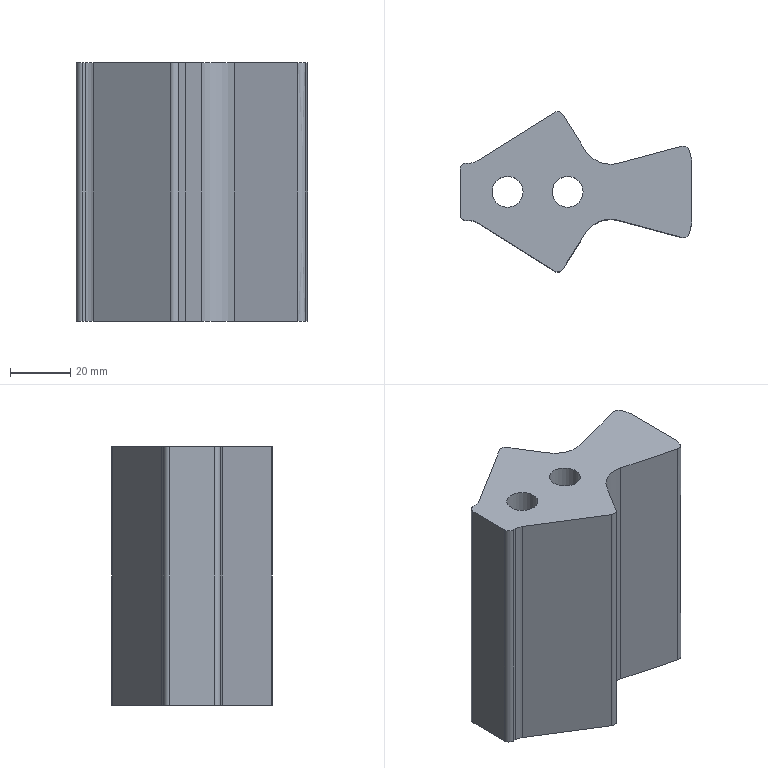Part | NX | features solid 2 | 1 solid | 34 faces | box 77 x 53.346 x 86 mm | volume 174595 mm3 | cylinder 14 | plane 14 | spline 6 | commonest cylinder face diameters 4 x4 10 x4 10.3 x2 17 x2 20 x2
STEP:
#1=CARTESIAN_POINT('',(1558.616,0.,32.));
#2=VERTEX_POINT('',#1);
#3=CARTESIAN_POINT('',(1567.116,0.,32.));
#4=DIRECTION('',(0.,0.,-1.));
#5=DIRECTION('',(-1.,0.,0.));
#6=AXIS2_PLACEMENT_3D('',#3,#4,#5);
#7=CIRCLE('',#6,8.5);
#8=EDGE_CURVE('',#2,#2,#7,.T.);
#9=ORIENTED_EDGE('',*,*,#8,.F.);
#10=EDGE_LOOP('',(#9));
#11=FACE_BOUND('',#10,.T.);
#12=CARTESIAN_POINT('',(1558.616,0.,-8.));
#13=VERTEX_POINT('',#12);
#14=CARTESIAN_POINT('',(1567.116,0.,-8.));
#15=DIRECTION('',(0.,0.,-1.));
#16=DIRECTION('',(-1.,0.,0.));
#17=AXIS2_PLACEMENT_3D('',#14,#15,#16);
#18=CIRCLE('',#17,8.5);
#19=EDGE_CURVE('',#13,#13,#18,.T.);
#20=ORIENTED_EDGE('',*,*,#19,.T.);
#21=EDGE_LOOP('',(#20));
#22=FACE_BOUND('',#21,.T.);
#23=CARTESIAN_POINT('',(1567.116,0.,-8.));
#24=DIRECTION('',(0.,0.,1.));
#25=DIRECTION('',(1.,0.,0.));
#26=AXIS2_PLACEMENT_3D('',#23,#24,#25);
#27=CYLINDRICAL_SURFACE('',#26,8.5);
#28=ADVANCED_FACE('',(#11,#22),#27,.F.);
#29=CARTESIAN_POINT('',(1561.966,0.,32.));
#30=VERTEX_POINT('',#29);
#31=CARTESIAN_POINT('',(1567.116,0.,32.));
#32=DIRECTION('',(0.,0.,-1.));
#33=DIRECTION('',(-1.,0.,0.));
#34=AXIS2_PLACEMENT_3D('',#31,#32,#33);
#35=CIRCLE('',#34,5.15);
#36=EDGE_CURVE('',#30,#30,#35,.T.);
#37=ORIENTED_EDGE('',*,*,#36,.F.);
#38=EDGE_LOOP('',(#37));
#39=FACE_BOUND('',#38,.T.);
#40=ORIENTED_EDGE('',*,*,#8,.T.);
#41=EDGE_LOOP('',(#40));
#42=FACE_BOUND('',#41,.T.);
#43=CARTESIAN_POINT('',(1094.146,58.387,32.));
#44=DIRECTION('',(0.,0.,-1.));
#45=DIRECTION('',(-1.,0.,0.));
#46=AXIS2_PLACEMENT_3D('',#43,#44,#45);
#47=PLANE('',#46);
#48=ADVANCED_FACE('',(#39,#42),#47,.T.);
#49=CARTESIAN_POINT('',(1561.966,0.,78.));
#50=VERTEX_POINT('',#49);
#51=CARTESIAN_POINT('',(1567.116,0.,78.));
#52=DIRECTION('',(0.,0.,-1.));
#53=DIRECTION('',(-1.,0.,0.));
#54=AXIS2_PLACEMENT_3D('',#51,#52,#53);
#55=CIRCLE('',#54,5.15);
#56=EDGE_CURVE('',#50,#50,#55,.F.);
#57=ORIENTED_EDGE('',*,*,#56,.T.);
#58=EDGE_LOOP('',(#57));
#59=FACE_BOUND('',#58,.T.);
#60=ORIENTED_EDGE('',*,*,#36,.T.);
#61=EDGE_LOOP('',(#60));
#62=FACE_BOUND('',#61,.T.);
#63=CARTESIAN_POINT('',(1567.116,0.,27.));
#64=DIRECTION('',(0.,0.,1.));
#65=DIRECTION('',(1.,0.,0.));
#66=AXIS2_PLACEMENT_3D('',#63,#64,#65);
#67=CYLINDRICAL_SURFACE('',#66,5.15);
#68=ADVANCED_FACE('',(#59,#62),#67,.F.);
#69=CARTESIAN_POINT('',(1541.966,0.,32.));
#70=VERTEX_POINT('',#69);
#71=CARTESIAN_POINT('',(1547.116,0.,32.));
#72=DIRECTION('',(0.,0.,-1.));
#73=DIRECTION('',(-1.,0.,0.));
#74=AXIS2_PLACEMENT_3D('',#71,#72,#73);
#75=CIRCLE('',#74,5.15);
#76=EDGE_CURVE('',#70,#70,#75,.T.);
#77=ORIENTED_EDGE('',*,*,#76,.F.);
#78=EDGE_LOOP('',(#77));
#79=FACE_BOUND('',#78,.T.);
#80=CARTESIAN_POINT('',(1538.616,0.,32.));
#81=VERTEX_POINT('',#80);
#82=CARTESIAN_POINT('',(1547.116,0.,32.));
#83=DIRECTION('',(0.,0.,-1.));
#84=DIRECTION('',(-1.,0.,0.));
#85=AXIS2_PLACEMENT_3D('',#82,#83,#84);
#86=CIRCLE('',#85,8.5);
#87=EDGE_CURVE('',#81,#81,#86,.T.);
#88=ORIENTED_EDGE('',*,*,#87,.T.);
#89=EDGE_LOOP('',(#88));
#90=FACE_BOUND('',#89,.T.);
#91=CARTESIAN_POINT('',(1074.146,58.387,32.));
#92=DIRECTION('',(0.,0.,-1.));
#93=DIRECTION('',(-1.,0.,0.));
#94=AXIS2_PLACEMENT_3D('',#91,#92,#93);
#95=PLANE('',#94);
#96=ADVANCED_FACE('',(#79,#90),#95,.T.);
#97=CARTESIAN_POINT('',(1541.966,0.,78.));
#98=VERTEX_POINT('',#97);
#99=CARTESIAN_POINT('',(1547.116,0.,78.));
#100=DIRECTION('',(0.,0.,-1.));
#101=DIRECTION('',(-1.,0.,0.));
#102=AXIS2_PLACEMENT_3D('',#99,#100,#101);
#103=CIRCLE('',#102,5.15);
#104=EDGE_CURVE('',#98,#98,#103,.T.);
#105=ORIENTED_EDGE('',*,*,#104,.F.);
#106=EDGE_LOOP('',(#105));
#107=FACE_BOUND('',#106,.T.);
#108=ORIENTED_EDGE('',*,*,#76,.T.);
#109=EDGE_LOOP('',(#108));
#110=FACE_BOUND('',#109,.T.);
#111=CARTESIAN_POINT('',(1547.116,0.,27.));
#112=DIRECTION('',(0.,0.,1.));
#113=DIRECTION('',(1.,0.,0.));
#114=AXIS2_PLACEMENT_3D('',#111,#112,#113);
#115=CYLINDRICAL_SURFACE('',#114,5.15);
#116=ADVANCED_FACE('',(#107,#110),#115,.F.);
#117=CARTESIAN_POINT('',(1608.226,11.348,-8.));
#118=VERTEX_POINT('',#117);
#119=CARTESIAN_POINT('',(1608.396,10.054,-8.));
#120=VERTEX_POINT('',#119);
#121=CARTESIAN_POINT('',(1603.396,10.054,-8.));
#122=DIRECTION('',(0.,0.,-1.));
#123=DIRECTION('',(-1.,0.,0.));
#124=AXIS2_PLACEMENT_3D('',#121,#122,#123);
#125=CIRCLE('',#124,5.);
#126=EDGE_CURVE('',#118,#120,#125,.T.);
#127=ORIENTED_EDGE('',*,*,#126,.F.);
#128=CARTESIAN_POINT('',(1608.226,11.348,78.));
#129=VERTEX_POINT('',#128);
#130=CARTESIAN_POINT('',(1608.226,11.348,-8.));
#131=DIRECTION('',(0.,0.,1.));
#132=VECTOR('',#131,1000.);
#133=LINE('',#130,#132);
#134=EDGE_CURVE('',#129,#118,#133,.F.);
#135=ORIENTED_EDGE('',*,*,#134,.F.);
#136=CARTESIAN_POINT('',(1608.396,10.054,78.));
#137=VERTEX_POINT('',#136);
#138=CARTESIAN_POINT('',(1603.396,10.054,78.));
#139=DIRECTION('',(0.,0.,-1.));
#140=DIRECTION('',(-1.,0.,0.));
#141=AXIS2_PLACEMENT_3D('',#138,#139,#140);
#142=CIRCLE('',#141,5.);
#143=EDGE_CURVE('',#137,#129,#142,.F.);
#144=ORIENTED_EDGE('',*,*,#143,.F.);
#145=CARTESIAN_POINT('',(1608.396,10.054,82.));
#146=DIRECTION('',(0.,0.,1.));
#147=VECTOR('',#146,1000.);
#148=LINE('',#145,#147);
#149=EDGE_CURVE('',#120,#137,#148,.T.);
#150=ORIENTED_EDGE('',*,*,#149,.F.);
#151=EDGE_LOOP('',(#127,#135,#144,#150));
#152=FACE_BOUND('',#151,.T.);
#153=CARTESIAN_POINT('',(1603.396,10.054,37.));
#154=DIRECTION('',(0.,0.,-1.));
#155=DIRECTION('',(-1.,0.,0.));
#156=AXIS2_PLACEMENT_3D('',#153,#154,#155);
#157=CYLINDRICAL_SURFACE('',#156,5.);
#158=ADVANCED_FACE('',(#152),#157,.T.);
#159=CARTESIAN_POINT('',(1607.583,13.748,78.));
#160=VERTEX_POINT('',#159);
#161=CARTESIAN_POINT('',(1602.079,34.289,78.));
#162=DIRECTION('',(-0.2588,0.9659,0.));
#163=VECTOR('',#162,1000.);
#164=LINE('',#161,#163);
#165=EDGE_CURVE('',#160,#129,#164,.F.);
#166=ORIENTED_EDGE('',*,*,#165,.T.);
#167=ORIENTED_EDGE('',*,*,#134,.T.);
#168=CARTESIAN_POINT('',(1607.583,13.748,-8.));
#169=VERTEX_POINT('',#168);
#170=CARTESIAN_POINT('',(1590.721,76.679,-8.));
#171=DIRECTION('',(0.2588,-0.9659,0.));
#172=VECTOR('',#171,1000.);
#173=LINE('',#170,#172);
#174=EDGE_CURVE('',#169,#118,#173,.T.);
#175=ORIENTED_EDGE('',*,*,#174,.F.);
#176=CARTESIAN_POINT('',(1607.583,13.748,-8.));
#177=CARTESIAN_POINT('',(1607.583,13.748,20.667));
#178=CARTESIAN_POINT('',(1607.583,13.748,49.333));
#179=CARTESIAN_POINT('',(1607.583,13.748,78.));
#180=B_SPLINE_CURVE_WITH_KNOTS('',3,(#176,#177,#178,#179),.UNSPECIFIED.,.F.,.F.,(4,4),(0.,0.086),.UNSPECIFIED.);
#181=EDGE_CURVE('',#169,#160,#180,.T.);
#182=ORIENTED_EDGE('',*,*,#181,.T.);
#183=EDGE_LOOP('',(#166,#167,#175,#182));
#184=FACE_BOUND('',#183,.T.);
#185=CARTESIAN_POINT('',(1602.079,34.289,84.));
#186=DIRECTION('',(0.9659,0.2588,0.));
#187=DIRECTION('',(-0.2588,0.9659,0.));
#188=AXIS2_PLACEMENT_3D('',#185,#186,#187);
#189=PLANE('',#188);
#190=ADVANCED_FACE('',(#184),#189,.T.);
#191=CARTESIAN_POINT('',(1605.133,15.163,-8.));
#192=VERTEX_POINT('',#191);
#193=CARTESIAN_POINT('',(1605.651,13.231,-8.));
#194=DIRECTION('',(0.,0.,-1.));
#195=DIRECTION('',(-1.,0.,0.));
#196=AXIS2_PLACEMENT_3D('',#193,#194,#195);
#197=CIRCLE('',#196,2.);
#198=EDGE_CURVE('',#192,#169,#197,.T.);
#199=ORIENTED_EDGE('',*,*,#198,.F.);
#200=CARTESIAN_POINT('',(1605.133,15.163,78.));
#201=VERTEX_POINT('',#200);
#202=CARTESIAN_POINT('',(1605.133,15.163,78.));
#203=CARTESIAN_POINT('',(1605.133,15.163,49.333));
#204=CARTESIAN_POINT('',(1605.133,15.163,20.667));
#205=CARTESIAN_POINT('',(1605.133,15.163,-8.));
#206=B_SPLINE_CURVE_WITH_KNOTS('',3,(#202,#203,#204,#205),.UNSPECIFIED.,.F.,.F.,(4,4),(0.004,0.09),.UNSPECIFIED.);
#207=EDGE_CURVE('',#201,#192,#206,.T.);
#208=ORIENTED_EDGE('',*,*,#207,.F.);
#209=CARTESIAN_POINT('',(1605.651,13.231,78.));
#210=DIRECTION('',(0.,0.,-1.));
#211=DIRECTION('',(-1.,0.,0.));
#212=AXIS2_PLACEMENT_3D('',#209,#210,#211);
#213=CIRCLE('',#212,2.);
#214=EDGE_CURVE('',#160,#201,#213,.F.);
#215=ORIENTED_EDGE('',*,*,#214,.F.);
#216=ORIENTED_EDGE('',*,*,#181,.F.);
#217=EDGE_LOOP('',(#199,#208,#215,#216));
#218=FACE_BOUND('',#217,.T.);
#219=CARTESIAN_POINT('',(1607.583,13.748,78.));
#220=CARTESIAN_POINT('',(1607.065,15.68,78.));
#221=CARTESIAN_POINT('',(1605.133,15.163,78.));
#222=CARTESIAN_POINT('',(1607.583,13.748,49.333));
#223=CARTESIAN_POINT('',(1607.065,15.68,49.333));
#224=CARTESIAN_POINT('',(1605.133,15.163,49.333));
#225=CARTESIAN_POINT('',(1607.583,13.748,20.667));
#226=CARTESIAN_POINT('',(1607.065,15.68,20.667));
#227=CARTESIAN_POINT('',(1605.133,15.163,20.667));
#228=CARTESIAN_POINT('',(1607.583,13.748,-8.));
#229=CARTESIAN_POINT('',(1607.065,15.68,-8.));
#230=CARTESIAN_POINT('',(1605.133,15.163,-8.));
#231=(BOUNDED_SURFACE()B_SPLINE_SURFACE(3,2,((#219,#220,#221),(#222,#223,#224),(#225,#226,#227),(#228,#229,#230)),.UNSPECIFIED.,.F.,.F.,.F.)B_SPLINE_SURFACE_WITH_KNOTS((4,4),(3,3),(0.1021,0.1881),(0.,1.),.PIECEWISE_BEZIER_KNOTS.)GEOMETRIC_REPRESENTATION_ITEM()RATIONAL_B_SPLINE_SURFACE(((1.,0.7071,1.),(1.,0.7071,1.),(1.,0.7071,1.),(1.,0.7071,1.)))REPRESENTATION_ITEM('')SURFACE());
#232=ADVANCED_FACE('',(#218),#231,.T.);
#233=CARTESIAN_POINT('',(1584.,9.5,78.));
#234=VERTEX_POINT('',#233);
#235=CARTESIAN_POINT('',(1605.133,15.163,78.));
#236=CARTESIAN_POINT('',(1598.089,13.275,78.));
#237=CARTESIAN_POINT('',(1591.044,11.388,78.));
#238=CARTESIAN_POINT('',(1584.,9.5,78.));
#239=B_SPLINE_CURVE_WITH_KNOTS('',3,(#235,#236,#237,#238),.UNSPECIFIED.,.F.,.F.,(4,4),(0.,0.02188),.UNSPECIFIED.);
#240=EDGE_CURVE('',#201,#234,#239,.T.);
#241=ORIENTED_EDGE('',*,*,#240,.F.);
#242=ORIENTED_EDGE('',*,*,#207,.T.);
#243=CARTESIAN_POINT('',(1584.,9.5,-8.));
#244=VERTEX_POINT('',#243);
#245=CARTESIAN_POINT('',(1584.,9.5,-8.));
#246=CARTESIAN_POINT('',(1591.044,11.388,-8.));
#247=CARTESIAN_POINT('',(1598.089,13.275,-8.));
#248=CARTESIAN_POINT('',(1605.133,15.163,-8.));
#249=B_SPLINE_CURVE_WITH_KNOTS('',3,(#245,#246,#247,#248),.UNSPECIFIED.,.F.,.F.,(4,4),(0.,0.02188),.UNSPECIFIED.);
#250=EDGE_CURVE('',#244,#192,#249,.T.);
#251=ORIENTED_EDGE('',*,*,#250,.F.);
#252=CARTESIAN_POINT('',(1584.,9.5,-1.));
#253=DIRECTION('',(0.000000369,0.000000231,1.));
#254=VECTOR('',#253,1000.);
#255=LINE('',#252,#254);
#256=EDGE_CURVE('',#234,#244,#255,.F.);
#257=ORIENTED_EDGE('',*,*,#256,.F.);
#258=EDGE_LOOP('',(#241,#242,#251,#257));
#259=FACE_BOUND('',#258,.T.);
#260=CARTESIAN_POINT('',(1584.,9.5,-8.));
#261=CARTESIAN_POINT('',(1584.,9.5,78.));
#262=CARTESIAN_POINT('',(1594.63,12.348,-8.));
#263=CARTESIAN_POINT('',(1594.63,12.348,78.));
#264=CARTESIAN_POINT('',(1605.26,15.197,-8.));
#265=CARTESIAN_POINT('',(1605.26,15.197,78.));
#266=B_SPLINE_SURFACE_WITH_KNOTS('',2,1,((#260,#261),(#262,#263),(#264,#265)),.SURF_OF_LINEAR_EXTRUSION.,.F.,.F.,.F.,(3,3),(2,2),(0.,0.8673),(0.,1.),.PIECEWISE_BEZIER_KNOTS.);
#267=ADVANCED_FACE('',(#259),#266,.F.);
#268=CARTESIAN_POINT('',(1572.931,13.86,-8.));
#269=VERTEX_POINT('',#268);
#270=CARTESIAN_POINT('',(1581.412,19.159,-8.));
#271=DIRECTION('',(0.,0.,-1.));
#272=DIRECTION('',(-1.,0.,0.));
#273=AXIS2_PLACEMENT_3D('',#270,#271,#272);
#274=CIRCLE('',#273,10.);
#275=EDGE_CURVE('',#269,#244,#274,.F.);
#276=ORIENTED_EDGE('',*,*,#275,.F.);
#277=CARTESIAN_POINT('',(1572.931,13.86,78.));
#278=VERTEX_POINT('',#277);
#279=CARTESIAN_POINT('',(1572.931,13.86,-4.));
#280=DIRECTION('',(0.000000369,0.000000231,1.));
#281=VECTOR('',#280,1000.);
#282=LINE('',#279,#281);
#283=EDGE_CURVE('',#269,#278,#282,.T.);
#284=ORIENTED_EDGE('',*,*,#283,.T.);
#285=CARTESIAN_POINT('',(1581.412,19.159,78.));
#286=DIRECTION('',(0.,0.,-1.));
#287=DIRECTION('',(-1.,0.,0.));
#288=AXIS2_PLACEMENT_3D('',#285,#286,#287);
#289=CIRCLE('',#288,10.);
#290=EDGE_CURVE('',#234,#278,#289,.T.);
#291=ORIENTED_EDGE('',*,*,#290,.F.);
#292=ORIENTED_EDGE('',*,*,#256,.T.);
#293=EDGE_LOOP('',(#276,#284,#291,#292));
#294=FACE_BOUND('',#293,.T.);
#295=CARTESIAN_POINT('',(1581.412,19.159,-2.5));
#296=DIRECTION('',(0.000000369,0.000000231,1.));
#297=DIRECTION('',(1.,0.,-0.000000369));
#298=AXIS2_PLACEMENT_3D('',#295,#296,#297);
#299=CYLINDRICAL_SURFACE('',#298,10.);
#300=ADVANCED_FACE('',(#294),#299,.F.);
#301=CARTESIAN_POINT('',(1567.632,22.341,78.));
#302=VERTEX_POINT('',#301);
#303=CARTESIAN_POINT('',(1567.632,22.341,-8.));
#304=VERTEX_POINT('',#303);
#305=CARTESIAN_POINT('',(1567.632,22.341,37.));
#306=DIRECTION('',(0.000000369,0.000000231,1.));
#307=VECTOR('',#306,1000.);
#308=LINE('',#305,#307);
#309=EDGE_CURVE('',#302,#304,#308,.F.);
#310=ORIENTED_EDGE('',*,*,#309,.F.);
#311=CARTESIAN_POINT('',(1572.931,13.86,78.));
#312=CARTESIAN_POINT('',(1571.165,16.687,78.));
#313=CARTESIAN_POINT('',(1569.399,19.514,78.));
#314=CARTESIAN_POINT('',(1567.632,22.341,78.));
#315=B_SPLINE_CURVE_WITH_KNOTS('',3,(#311,#312,#313,#314),.UNSPECIFIED.,.F.,.F.,(4,4),(0.,0.01),.UNSPECIFIED.);
#316=EDGE_CURVE('',#278,#302,#315,.T.);
#317=ORIENTED_EDGE('',*,*,#316,.F.);
#318=ORIENTED_EDGE('',*,*,#283,.F.);
#319=CARTESIAN_POINT('',(1567.632,22.341,-8.));
#320=CARTESIAN_POINT('',(1569.399,19.514,-8.));
#321=CARTESIAN_POINT('',(1571.165,16.687,-8.));
#322=CARTESIAN_POINT('',(1572.931,13.86,-8.));
#323=B_SPLINE_CURVE_WITH_KNOTS('',3,(#319,#320,#321,#322),.UNSPECIFIED.,.F.,.F.,(4,4),(0.,0.01),.UNSPECIFIED.);
#324=EDGE_CURVE('',#304,#269,#323,.T.);
#325=ORIENTED_EDGE('',*,*,#324,.F.);
#326=EDGE_LOOP('',(#310,#317,#318,#325));
#327=FACE_BOUND('',#326,.T.);
#328=CARTESIAN_POINT('',(1567.632,22.341,-8.));
#329=CARTESIAN_POINT('',(1567.632,22.341,78.));
#330=CARTESIAN_POINT('',(1570.282,18.1,-8.));
#331=CARTESIAN_POINT('',(1570.282,18.1,78.));
#332=CARTESIAN_POINT('',(1572.931,13.86,-8.));
#333=CARTESIAN_POINT('',(1572.931,13.86,78.));
#334=B_SPLINE_SURFACE_WITH_KNOTS('',2,1,((#328,#329),(#330,#331),(#332,#333)),.SURF_OF_LINEAR_EXTRUSION.,.F.,.F.,.F.,(3,3),(2,2),(0.8758,1.),(0.,1.),.PIECEWISE_BEZIER_KNOTS.);
#335=ADVANCED_FACE('',(#327),#334,.F.);
#336=CARTESIAN_POINT('',(1565.512,25.733,-8.));
#337=VERTEX_POINT('',#336);
#338=CARTESIAN_POINT('',(1468.843,180.436,-8.));
#339=DIRECTION('',(0.5299,-0.848,0.));
#340=VECTOR('',#339,1000.);
#341=LINE('',#338,#340);
#342=EDGE_CURVE('',#337,#304,#341,.T.);
#343=ORIENTED_EDGE('',*,*,#342,.F.);
#344=CARTESIAN_POINT('',(1565.512,25.733,78.));
#345=VERTEX_POINT('',#344);
#346=CARTESIAN_POINT('',(1565.512,25.733,37.));
#347=DIRECTION('',(-0.000000369,-0.000000231,-1.));
#348=VECTOR('',#347,1000.);
#349=LINE('',#346,#348);
#350=EDGE_CURVE('',#337,#345,#349,.F.);
#351=ORIENTED_EDGE('',*,*,#350,.T.);
#352=CARTESIAN_POINT('',(1567.632,22.341,78.));
#353=DIRECTION('',(-0.5299,0.848,0.));
#354=VECTOR('',#353,1000.);
#355=LINE('',#352,#354);
#356=EDGE_CURVE('',#345,#302,#355,.F.);
#357=ORIENTED_EDGE('',*,*,#356,.T.);
#358=ORIENTED_EDGE('',*,*,#309,.T.);
#359=EDGE_LOOP('',(#343,#351,#357,#358));
#360=FACE_BOUND('',#359,.T.);
#361=CARTESIAN_POINT('',(1567.632,22.341,37.));
#362=DIRECTION('',(0.848,0.5299,-0.000000435));
#363=DIRECTION('',(-0.5299,0.848,0.));
#364=AXIS2_PLACEMENT_3D('',#361,#362,#363);
#365=PLANE('',#364);
#366=ADVANCED_FACE('',(#360),#365,.T.);
#367=CARTESIAN_POINT('',(1562.757,26.369,78.));
#368=VERTEX_POINT('',#367);
#369=CARTESIAN_POINT('',(1563.816,24.673,78.));
#370=DIRECTION('',(0.,0.,-1.));
#371=DIRECTION('',(-1.,0.,0.));
#372=AXIS2_PLACEMENT_3D('',#369,#370,#371);
#373=CIRCLE('',#372,2.);
#374=EDGE_CURVE('',#345,#368,#373,.F.);
#375=ORIENTED_EDGE('',*,*,#374,.F.);
#376=ORIENTED_EDGE('',*,*,#350,.F.);
#377=CARTESIAN_POINT('',(1562.757,26.369,-8.));
#378=VERTEX_POINT('',#377);
#379=CARTESIAN_POINT('',(1563.816,24.673,-8.));
#380=DIRECTION('',(0.,0.,-1.));
#381=DIRECTION('',(-1.,0.,0.));
#382=AXIS2_PLACEMENT_3D('',#379,#380,#381);
#383=CIRCLE('',#382,2.);
#384=EDGE_CURVE('',#378,#337,#383,.T.);
#385=ORIENTED_EDGE('',*,*,#384,.F.);
#386=CARTESIAN_POINT('',(1562.757,26.369,29.227));
#387=DIRECTION('',(-0.000000369,-0.000000231,-1.));
#388=VECTOR('',#387,1000.);
#389=LINE('',#386,#388);
#390=EDGE_CURVE('',#368,#378,#389,.T.);
#391=ORIENTED_EDGE('',*,*,#390,.F.);
#392=EDGE_LOOP('',(#375,#376,#385,#391));
#393=FACE_BOUND('',#392,.T.);
#394=CARTESIAN_POINT('',(1563.816,24.673,29.227));
#395=DIRECTION('',(-0.000000369,-0.000000231,-1.));
#396=DIRECTION('',(-1.,0.,0.000000369));
#397=AXIS2_PLACEMENT_3D('',#394,#395,#396);
#398=CYLINDRICAL_SURFACE('',#397,2.);
#399=ADVANCED_FACE('',(#393),#398,.T.);
#400=CARTESIAN_POINT('',(1536.976,10.26,-8.));
#401=VERTEX_POINT('',#400);
#402=CARTESIAN_POINT('',(1182.255,-211.395,-8.));
#403=DIRECTION('',(0.848,0.5299,0.));
#404=VECTOR('',#403,1000.);
#405=LINE('',#402,#404);
#406=EDGE_CURVE('',#401,#378,#405,.T.);
#407=ORIENTED_EDGE('',*,*,#406,.F.);
#408=CARTESIAN_POINT('',(1536.976,10.26,78.));
#409=VERTEX_POINT('',#408);
#410=CARTESIAN_POINT('',(1536.976,10.26,82.));
#411=DIRECTION('',(0.,0.,1.));
#412=VECTOR('',#411,1000.);
#413=LINE('',#410,#412);
#414=EDGE_CURVE('',#401,#409,#413,.T.);
#415=ORIENTED_EDGE('',*,*,#414,.T.);
#416=CARTESIAN_POINT('',(1999.247,299.119,78.));
#417=DIRECTION('',(0.848,0.5299,0.));
#418=VECTOR('',#417,1000.);
#419=LINE('',#416,#418);
#420=EDGE_CURVE('',#368,#409,#419,.F.);
#421=ORIENTED_EDGE('',*,*,#420,.F.);
#422=ORIENTED_EDGE('',*,*,#390,.T.);
#423=EDGE_LOOP('',(#407,#415,#421,#422));
#424=FACE_BOUND('',#423,.T.);
#425=CARTESIAN_POINT('',(1636.537,72.472,29.227));
#426=DIRECTION('',(-0.5299,0.848,0.));
#427=DIRECTION('',(-0.848,-0.5299,0.));
#428=AXIS2_PLACEMENT_3D('',#425,#426,#427);
#429=PLANE('',#428);
#430=ADVANCED_FACE('',(#424),#429,.T.);
#431=CARTESIAN_POINT('',(1534.327,9.5,78.));
#432=VERTEX_POINT('',#431);
#433=CARTESIAN_POINT('',(1534.327,14.5,78.));
#434=DIRECTION('',(0.,0.,-1.));
#435=DIRECTION('',(-1.,0.,0.));
#436=AXIS2_PLACEMENT_3D('',#433,#434,#435);
#437=CIRCLE('',#436,5.);
#438=EDGE_CURVE('',#409,#432,#437,.T.);
#439=ORIENTED_EDGE('',*,*,#438,.F.);
#440=ORIENTED_EDGE('',*,*,#414,.F.);
#441=CARTESIAN_POINT('',(1534.327,9.5,-8.));
#442=VERTEX_POINT('',#441);
#443=CARTESIAN_POINT('',(1534.327,14.5,-8.));
#444=DIRECTION('',(0.,0.,-1.));
#445=DIRECTION('',(-1.,0.,0.));
#446=AXIS2_PLACEMENT_3D('',#443,#444,#445);
#447=CIRCLE('',#446,5.);
#448=EDGE_CURVE('',#442,#401,#447,.F.);
#449=ORIENTED_EDGE('',*,*,#448,.F.);
#450=CARTESIAN_POINT('',(1534.327,9.5,-8.));
#451=DIRECTION('',(0.,0.,-1.));
#452=VECTOR('',#451,1000.);
#453=LINE('',#450,#452);
#454=EDGE_CURVE('',#432,#442,#453,.T.);
#455=ORIENTED_EDGE('',*,*,#454,.F.);
#456=EDGE_LOOP('',(#439,#440,#449,#455));
#457=FACE_BOUND('',#456,.T.);
#458=CARTESIAN_POINT('',(1534.327,14.5,0.));
#459=DIRECTION('',(0.,0.,-1.));
#460=DIRECTION('',(-1.,0.,0.));
#461=AXIS2_PLACEMENT_3D('',#458,#459,#460);
#462=CYLINDRICAL_SURFACE('',#461,5.);
#463=ADVANCED_FACE('',(#457),#462,.F.);
#464=CARTESIAN_POINT('',(1533.396,9.5,-8.));
#465=VERTEX_POINT('',#464);
#466=CARTESIAN_POINT('',(1086.646,9.5,-8.));
#467=DIRECTION('',(-1.,0.,0.));
#468=VECTOR('',#467,1000.);
#469=LINE('',#466,#468);
#470=EDGE_CURVE('',#465,#442,#469,.F.);
#471=ORIENTED_EDGE('',*,*,#470,.F.);
#472=CARTESIAN_POINT('',(1533.396,9.5,78.));
#473=VERTEX_POINT('',#472);
#474=CARTESIAN_POINT('',(1533.396,9.5,82.));
#475=DIRECTION('',(0.,0.,1.));
#476=VECTOR('',#475,1000.);
#477=LINE('',#474,#476);
#478=EDGE_CURVE('',#465,#473,#477,.T.);
#479=ORIENTED_EDGE('',*,*,#478,.T.);
#480=CARTESIAN_POINT('',(2186.158,9.5,78.));
#481=DIRECTION('',(-1.,0.,0.));
#482=VECTOR('',#481,1000.);
#483=LINE('',#480,#482);
#484=EDGE_CURVE('',#432,#473,#483,.T.);
#485=ORIENTED_EDGE('',*,*,#484,.F.);
#486=ORIENTED_EDGE('',*,*,#454,.T.);
#487=EDGE_LOOP('',(#471,#479,#485,#486));
#488=FACE_BOUND('',#487,.T.);
#489=CARTESIAN_POINT('',(984.466,9.5,0.));
#490=DIRECTION('',(0.,-1.,0.));
#491=DIRECTION('',(1.,0.,0.));
#492=AXIS2_PLACEMENT_3D('',#489,#490,#491);
#493=PLANE('',#492);
#494=ADVANCED_FACE('',(#488),#493,.F.);
#495=CARTESIAN_POINT('',(1531.396,7.5,78.));
#496=VERTEX_POINT('',#495);
#497=CARTESIAN_POINT('',(1533.396,7.5,78.));
#498=DIRECTION('',(0.,0.,-1.));
#499=DIRECTION('',(-1.,0.,0.));
#500=AXIS2_PLACEMENT_3D('',#497,#498,#499);
#501=CIRCLE('',#500,2.);
#502=EDGE_CURVE('',#473,#496,#501,.F.);
#503=ORIENTED_EDGE('',*,*,#502,.F.);
#504=ORIENTED_EDGE('',*,*,#478,.F.);
#505=CARTESIAN_POINT('',(1531.396,7.5,-8.));
#506=VERTEX_POINT('',#505);
#507=CARTESIAN_POINT('',(1533.396,7.5,-8.));
#508=DIRECTION('',(0.,0.,-1.));
#509=DIRECTION('',(-1.,0.,0.));
#510=AXIS2_PLACEMENT_3D('',#507,#508,#509);
#511=CIRCLE('',#510,2.);
#512=EDGE_CURVE('',#506,#465,#511,.T.);
#513=ORIENTED_EDGE('',*,*,#512,.F.);
#514=CARTESIAN_POINT('',(1531.396,7.5,-8.));
#515=DIRECTION('',(0.,0.,1.));
#516=VECTOR('',#515,1000.);
#517=LINE('',#514,#516);
#518=EDGE_CURVE('',#496,#506,#517,.F.);
#519=ORIENTED_EDGE('',*,*,#518,.F.);
#520=EDGE_LOOP('',(#503,#504,#513,#519));
#521=FACE_BOUND('',#520,.T.);
#522=CARTESIAN_POINT('',(1533.396,7.5,0.));
#523=DIRECTION('',(0.,0.,1.));
#524=DIRECTION('',(1.,0.,0.));
#525=AXIS2_PLACEMENT_3D('',#522,#523,#524);
#526=CYLINDRICAL_SURFACE('',#525,2.);
#527=ADVANCED_FACE('',(#521),#526,.T.);
#528=CARTESIAN_POINT('',(1531.396,-7.5,78.));
#529=VERTEX_POINT('',#528);
#530=CARTESIAN_POINT('',(1531.396,0.,78.));
#531=DIRECTION('',(0.,-1.,0.));
#532=VECTOR('',#531,1000.);
#533=LINE('',#530,#532);
#534=EDGE_CURVE('',#496,#529,#533,.T.);
#535=ORIENTED_EDGE('',*,*,#534,.F.);
#536=ORIENTED_EDGE('',*,*,#518,.T.);
#537=CARTESIAN_POINT('',(1531.396,-7.5,-8.));
#538=VERTEX_POINT('',#537);
#539=CARTESIAN_POINT('',(1531.396,58.387,-8.));
#540=DIRECTION('',(0.,-1.,0.));
#541=VECTOR('',#540,1000.);
#542=LINE('',#539,#541);
#543=EDGE_CURVE('',#506,#538,#542,.T.);
#544=ORIENTED_EDGE('',*,*,#543,.T.);
#545=CARTESIAN_POINT('',(1531.396,-7.5,-8.));
#546=DIRECTION('',(0.,0.,1.));
#547=VECTOR('',#546,1000.);
#548=LINE('',#545,#547);
#549=EDGE_CURVE('',#529,#538,#548,.F.);
#550=ORIENTED_EDGE('',*,*,#549,.F.);
#551=EDGE_LOOP('',(#535,#536,#544,#550));
#552=FACE_BOUND('',#551,.T.);
#553=CARTESIAN_POINT('',(1531.396,0.,0.));
#554=DIRECTION('',(-1.,0.,0.));
#555=DIRECTION('',(0.,-1.,0.));
#556=AXIS2_PLACEMENT_3D('',#553,#554,#555);
#557=PLANE('',#556);
#558=ADVANCED_FACE('',(#552),#557,.T.);
#559=CARTESIAN_POINT('',(1533.396,-9.5,78.));
#560=VERTEX_POINT('',#559);
#561=CARTESIAN_POINT('',(1533.396,-7.5,78.));
#562=DIRECTION('',(0.,0.,-1.));
#563=DIRECTION('',(-1.,0.,0.));
#564=AXIS2_PLACEMENT_3D('',#561,#562,#563);
#565=CIRCLE('',#564,2.);
#566=EDGE_CURVE('',#560,#529,#565,.T.);
#567=ORIENTED_EDGE('',*,*,#566,.T.);
#568=ORIENTED_EDGE('',*,*,#549,.T.);
#569=CARTESIAN_POINT('',(1533.396,-9.5,-8.));
#570=VERTEX_POINT('',#569);
#571=CARTESIAN_POINT('',(1533.396,-7.5,-8.));
#572=DIRECTION('',(0.,0.,1.));
#573=DIRECTION('',(-1.,0.,0.));
#574=AXIS2_PLACEMENT_3D('',#571,#572,#573);
#575=CIRCLE('',#574,2.);
#576=EDGE_CURVE('',#538,#570,#575,.T.);
#577=ORIENTED_EDGE('',*,*,#576,.T.);
#578=CARTESIAN_POINT('',(1533.396,-9.5,82.));
#579=DIRECTION('',(0.,0.,1.));
#580=VECTOR('',#579,1000.);
#581=LINE('',#578,#580);
#582=EDGE_CURVE('',#570,#560,#581,.T.);
#583=ORIENTED_EDGE('',*,*,#582,.T.);
#584=EDGE_LOOP('',(#567,#568,#577,#583));
#585=FACE_BOUND('',#584,.T.);
#586=CARTESIAN_POINT('',(1533.396,-7.5,0.));
#587=DIRECTION('',(0.,0.,1.));
#588=DIRECTION('',(1.,0.,0.));
#589=AXIS2_PLACEMENT_3D('',#586,#587,#588);
#590=CYLINDRICAL_SURFACE('',#589,2.);
#591=ADVANCED_FACE('',(#585),#590,.T.);
#592=CARTESIAN_POINT('',(1534.327,-9.5,-8.));
#593=VERTEX_POINT('',#592);
#594=CARTESIAN_POINT('',(1086.646,-9.5,-8.));
#595=DIRECTION('',(-1.,0.,0.));
#596=VECTOR('',#595,1000.);
#597=LINE('',#594,#596);
#598=EDGE_CURVE('',#570,#593,#597,.F.);
#599=ORIENTED_EDGE('',*,*,#598,.T.);
#600=CARTESIAN_POINT('',(1534.327,-9.5,78.));
#601=VERTEX_POINT('',#600);
#602=CARTESIAN_POINT('',(1534.327,-9.5,-8.));
#603=DIRECTION('',(0.,0.,-1.));
#604=VECTOR('',#603,1000.);
#605=LINE('',#602,#604);
#606=EDGE_CURVE('',#601,#593,#605,.T.);
#607=ORIENTED_EDGE('',*,*,#606,.F.);
#608=CARTESIAN_POINT('',(984.466,-9.5,78.));
#609=DIRECTION('',(-1.,0.,0.));
#610=VECTOR('',#609,1000.);
#611=LINE('',#608,#610);
#612=EDGE_CURVE('',#601,#560,#611,.T.);
#613=ORIENTED_EDGE('',*,*,#612,.T.);
#614=ORIENTED_EDGE('',*,*,#582,.F.);
#615=EDGE_LOOP('',(#599,#607,#613,#614));
#616=FACE_BOUND('',#615,.T.);
#617=CARTESIAN_POINT('',(984.466,-9.5,0.));
#618=DIRECTION('',(0.,1.,0.));
#619=DIRECTION('',(1.,0.,0.));
#620=AXIS2_PLACEMENT_3D('',#617,#618,#619);
#621=PLANE('',#620);
#622=ADVANCED_FACE('',(#616),#621,.F.);
#623=CARTESIAN_POINT('',(1536.976,-10.26,78.));
#624=VERTEX_POINT('',#623);
#625=CARTESIAN_POINT('',(1534.327,-14.5,78.));
#626=DIRECTION('',(0.,0.,-1.));
#627=DIRECTION('',(-1.,0.,0.));
#628=AXIS2_PLACEMENT_3D('',#625,#626,#627);
#629=CIRCLE('',#628,5.);
#630=EDGE_CURVE('',#624,#601,#629,.F.);
#631=ORIENTED_EDGE('',*,*,#630,.T.);
#632=ORIENTED_EDGE('',*,*,#606,.T.);
#633=CARTESIAN_POINT('',(1536.976,-10.26,-8.));
#634=VERTEX_POINT('',#633);
#635=CARTESIAN_POINT('',(1534.327,-14.5,-8.));
#636=DIRECTION('',(0.,0.,1.));
#637=DIRECTION('',(-1.,0.,0.));
#638=AXIS2_PLACEMENT_3D('',#635,#636,#637);
#639=CIRCLE('',#638,5.);
#640=EDGE_CURVE('',#593,#634,#639,.F.);
#641=ORIENTED_EDGE('',*,*,#640,.T.);
#642=CARTESIAN_POINT('',(1536.976,-10.26,82.));
#643=DIRECTION('',(0.,0.,1.));
#644=VECTOR('',#643,1000.);
#645=LINE('',#642,#644);
#646=EDGE_CURVE('',#634,#624,#645,.T.);
#647=ORIENTED_EDGE('',*,*,#646,.T.);
#648=EDGE_LOOP('',(#631,#632,#641,#647));
#649=FACE_BOUND('',#648,.T.);
#650=CARTESIAN_POINT('',(1534.327,-14.5,0.));
#651=DIRECTION('',(0.,0.,-1.));
#652=DIRECTION('',(-1.,0.,0.));
#653=AXIS2_PLACEMENT_3D('',#650,#651,#652);
#654=CYLINDRICAL_SURFACE('',#653,5.);
#655=ADVANCED_FACE('',(#649),#654,.F.);
#656=CARTESIAN_POINT('',(1562.757,-26.369,-8.));
#657=VERTEX_POINT('',#656);
#658=CARTESIAN_POINT('',(1182.255,211.395,-8.));
#659=DIRECTION('',(0.848,-0.5299,0.));
#660=VECTOR('',#659,1000.);
#661=LINE('',#658,#660);
#662=EDGE_CURVE('',#634,#657,#661,.T.);
#663=ORIENTED_EDGE('',*,*,#662,.T.);
#664=CARTESIAN_POINT('',(1562.757,-26.369,78.));
#665=VERTEX_POINT('',#664);
#666=CARTESIAN_POINT('',(1562.757,-26.369,29.227));
#667=DIRECTION('',(-0.000000369,0.000000231,-1.));
#668=VECTOR('',#667,1000.);
#669=LINE('',#666,#668);
#670=EDGE_CURVE('',#665,#657,#669,.T.);
#671=ORIENTED_EDGE('',*,*,#670,.F.);
#672=CARTESIAN_POINT('',(1636.537,-72.472,78.));
#673=DIRECTION('',(0.848,-0.5299,0.));
#674=VECTOR('',#673,1000.);
#675=LINE('',#672,#674);
#676=EDGE_CURVE('',#665,#624,#675,.F.);
#677=ORIENTED_EDGE('',*,*,#676,.T.);
#678=ORIENTED_EDGE('',*,*,#646,.F.);
#679=EDGE_LOOP('',(#663,#671,#677,#678));
#680=FACE_BOUND('',#679,.T.);
#681=CARTESIAN_POINT('',(1636.537,-72.472,29.227));
#682=DIRECTION('',(-0.5299,-0.848,0.));
#683=DIRECTION('',(-0.848,0.5299,0.));
#684=AXIS2_PLACEMENT_3D('',#681,#682,#683);
#685=PLANE('',#684);
#686=ADVANCED_FACE('',(#680),#685,.T.);
#687=CARTESIAN_POINT('',(1565.512,-25.733,78.));
#688=VERTEX_POINT('',#687);
#689=CARTESIAN_POINT('',(1563.816,-24.673,78.));
#690=DIRECTION('',(0.,0.,-1.));
#691=DIRECTION('',(-1.,0.,0.));
#692=AXIS2_PLACEMENT_3D('',#689,#690,#691);
#693=CIRCLE('',#692,2.);
#694=EDGE_CURVE('',#688,#665,#693,.T.);
#695=ORIENTED_EDGE('',*,*,#694,.T.);
#696=ORIENTED_EDGE('',*,*,#670,.T.);
#697=CARTESIAN_POINT('',(1565.512,-25.733,-8.));
#698=VERTEX_POINT('',#697);
#699=CARTESIAN_POINT('',(1563.816,-24.673,-8.));
#700=DIRECTION('',(0.,0.,1.));
#701=DIRECTION('',(-1.,0.,0.));
#702=AXIS2_PLACEMENT_3D('',#699,#700,#701);
#703=CIRCLE('',#702,2.);
#704=EDGE_CURVE('',#657,#698,#703,.T.);
#705=ORIENTED_EDGE('',*,*,#704,.T.);
#706=CARTESIAN_POINT('',(1565.512,-25.733,37.));
#707=DIRECTION('',(-0.000000369,0.000000231,-1.));
#708=VECTOR('',#707,1000.);
#709=LINE('',#706,#708);
#710=EDGE_CURVE('',#698,#688,#709,.F.);
#711=ORIENTED_EDGE('',*,*,#710,.T.);
#712=EDGE_LOOP('',(#695,#696,#705,#711));
#713=FACE_BOUND('',#712,.T.);
#714=CARTESIAN_POINT('',(1563.816,-24.673,29.227));
#715=DIRECTION('',(-0.000000369,0.000000231,-1.));
#716=DIRECTION('',(-1.,0.,0.000000369));
#717=AXIS2_PLACEMENT_3D('',#714,#715,#716);
#718=CYLINDRICAL_SURFACE('',#717,2.);
#719=ADVANCED_FACE('',(#713),#718,.T.);
#720=CARTESIAN_POINT('',(1567.632,-22.341,-8.));
#721=VERTEX_POINT('',#720);
#722=CARTESIAN_POINT('',(1468.843,-180.436,-8.));
#723=DIRECTION('',(0.5299,0.848,0.));
#724=VECTOR('',#723,1000.);
#725=LINE('',#722,#724);
#726=EDGE_CURVE('',#698,#721,#725,.T.);
#727=ORIENTED_EDGE('',*,*,#726,.T.);
#728=CARTESIAN_POINT('',(1567.632,-22.341,78.));
#729=VERTEX_POINT('',#728);
#730=CARTESIAN_POINT('',(1567.632,-22.341,37.));
#731=DIRECTION('',(0.000000369,-0.000000231,1.));
#732=VECTOR('',#731,1000.);
#733=LINE('',#730,#732);
#734=EDGE_CURVE('',#729,#721,#733,.F.);
#735=ORIENTED_EDGE('',*,*,#734,.F.);
#736=CARTESIAN_POINT('',(1751.363,271.69,78.));
#737=DIRECTION('',(-0.5299,-0.848,0.));
#738=VECTOR('',#737,1000.);
#739=LINE('',#736,#738);
#740=EDGE_CURVE('',#688,#729,#739,.F.);
#741=ORIENTED_EDGE('',*,*,#740,.F.);
#742=ORIENTED_EDGE('',*,*,#710,.F.);
#743=EDGE_LOOP('',(#727,#735,#741,#742));
#744=FACE_BOUND('',#743,.T.);
#745=CARTESIAN_POINT('',(1567.632,-22.341,37.));
#746=DIRECTION('',(0.848,-0.5299,-0.000000435));
#747=DIRECTION('',(-0.5299,-0.848,0.));
#748=AXIS2_PLACEMENT_3D('',#745,#746,#747);
#749=PLANE('',#748);
#750=ADVANCED_FACE('',(#744),#749,.T.);
#751=ORIENTED_EDGE('',*,*,#734,.T.);
#752=CARTESIAN_POINT('',(1572.931,-13.86,-8.));
#753=VERTEX_POINT('',#752);
#754=CARTESIAN_POINT('',(1567.632,-22.341,-8.));
#755=CARTESIAN_POINT('',(1569.399,-19.514,-8.));
#756=CARTESIAN_POINT('',(1571.165,-16.687,-8.));
#757=CARTESIAN_POINT('',(1572.931,-13.86,-8.));
#758=B_SPLINE_CURVE_WITH_KNOTS('',3,(#754,#755,#756,#757),.UNSPECIFIED.,.F.,.F.,(4,4),(0.,0.01),.UNSPECIFIED.);
#759=EDGE_CURVE('',#721,#753,#758,.T.);
#760=ORIENTED_EDGE('',*,*,#759,.T.);
#761=CARTESIAN_POINT('',(1572.931,-13.86,78.));
#762=VERTEX_POINT('',#761);
#763=CARTESIAN_POINT('',(1572.931,-13.86,-4.));
#764=DIRECTION('',(0.000000369,-0.000000231,1.));
#765=VECTOR('',#764,1000.);
#766=LINE('',#763,#765);
#767=EDGE_CURVE('',#753,#762,#766,.T.);
#768=ORIENTED_EDGE('',*,*,#767,.T.);
#769=CARTESIAN_POINT('',(1572.931,-13.86,78.));
#770=CARTESIAN_POINT('',(1571.165,-16.687,78.));
#771=CARTESIAN_POINT('',(1569.399,-19.514,78.));
#772=CARTESIAN_POINT('',(1567.632,-22.341,78.));
#773=B_SPLINE_CURVE_WITH_KNOTS('',3,(#769,#770,#771,#772),.UNSPECIFIED.,.F.,.F.,(4,4),(0.,0.01),.UNSPECIFIED.);
#774=EDGE_CURVE('',#762,#729,#773,.T.);
#775=ORIENTED_EDGE('',*,*,#774,.T.);
#776=EDGE_LOOP('',(#751,#760,#768,#775));
#777=FACE_BOUND('',#776,.T.);
#778=CARTESIAN_POINT('',(1567.632,-22.341,-8.));
#779=CARTESIAN_POINT('',(1567.632,-22.341,78.));
#780=CARTESIAN_POINT('',(1570.282,-18.1,-8.));
#781=CARTESIAN_POINT('',(1570.282,-18.1,78.));
#782=CARTESIAN_POINT('',(1572.931,-13.86,-8.));
#783=CARTESIAN_POINT('',(1572.931,-13.86,78.));
#784=B_SPLINE_SURFACE_WITH_KNOTS('',2,1,((#778,#779),(#780,#781),(#782,#783)),.SURF_OF_LINEAR_EXTRUSION.,.F.,.F.,.F.,(3,3),(2,2),(0.8758,1.),(0.,1.),.PIECEWISE_BEZIER_KNOTS.);
#785=ADVANCED_FACE('',(#777),#784,.T.);
#786=CARTESIAN_POINT('',(1584.,-9.5,-8.));
#787=VERTEX_POINT('',#786);
#788=CARTESIAN_POINT('',(1581.412,-19.159,-8.));
#789=DIRECTION('',(0.,0.,1.));
#790=DIRECTION('',(-1.,0.,0.));
#791=AXIS2_PLACEMENT_3D('',#788,#789,#790);
#792=CIRCLE('',#791,10.);
#793=EDGE_CURVE('',#753,#787,#792,.F.);
#794=ORIENTED_EDGE('',*,*,#793,.T.);
#795=CARTESIAN_POINT('',(1584.,-9.5,78.));
#796=VERTEX_POINT('',#795);
#797=CARTESIAN_POINT('',(1584.,-9.5,-1.));
#798=DIRECTION('',(0.000000369,-0.000000231,1.));
#799=VECTOR('',#798,1000.);
#800=LINE('',#797,#799);
#801=EDGE_CURVE('',#796,#787,#800,.F.);
#802=ORIENTED_EDGE('',*,*,#801,.F.);
#803=CARTESIAN_POINT('',(1581.412,-19.159,78.));
#804=DIRECTION('',(0.,0.,-1.));
#805=DIRECTION('',(-1.,0.,0.));
#806=AXIS2_PLACEMENT_3D('',#803,#804,#805);
#807=CIRCLE('',#806,10.);
#808=EDGE_CURVE('',#796,#762,#807,.F.);
#809=ORIENTED_EDGE('',*,*,#808,.T.);
#810=ORIENTED_EDGE('',*,*,#767,.F.);
#811=EDGE_LOOP('',(#794,#802,#809,#810));
#812=FACE_BOUND('',#811,.T.);
#813=CARTESIAN_POINT('',(1581.412,-19.159,-2.5));
#814=DIRECTION('',(0.000000369,-0.000000231,1.));
#815=DIRECTION('',(1.,0.,-0.000000369));
#816=AXIS2_PLACEMENT_3D('',#813,#814,#815);
#817=CYLINDRICAL_SURFACE('',#816,10.);
#818=ADVANCED_FACE('',(#812),#817,.F.);
#819=CARTESIAN_POINT('',(1605.133,-15.163,78.));
#820=VERTEX_POINT('',#819);
#821=CARTESIAN_POINT('',(1605.133,-15.163,78.));
#822=CARTESIAN_POINT('',(1598.089,-13.275,78.));
#823=CARTESIAN_POINT('',(1591.044,-11.388,78.));
#824=CARTESIAN_POINT('',(1584.,-9.5,78.));
#825=B_SPLINE_CURVE_WITH_KNOTS('',3,(#821,#822,#823,#824),.UNSPECIFIED.,.F.,.F.,(4,4),(0.,0.02188),.UNSPECIFIED.);
#826=EDGE_CURVE('',#820,#796,#825,.T.);
#827=ORIENTED_EDGE('',*,*,#826,.T.);
#828=ORIENTED_EDGE('',*,*,#801,.T.);
#829=CARTESIAN_POINT('',(1605.133,-15.163,-8.));
#830=VERTEX_POINT('',#829);
#831=CARTESIAN_POINT('',(1584.,-9.5,-8.));
#832=CARTESIAN_POINT('',(1591.044,-11.388,-8.));
#833=CARTESIAN_POINT('',(1598.089,-13.275,-8.));
#834=CARTESIAN_POINT('',(1605.133,-15.163,-8.));
#835=B_SPLINE_CURVE_WITH_KNOTS('',3,(#831,#832,#833,#834),.UNSPECIFIED.,.F.,.F.,(4,4),(0.,0.02188),.UNSPECIFIED.);
#836=EDGE_CURVE('',#787,#830,#835,.T.);
#837=ORIENTED_EDGE('',*,*,#836,.T.);
#838=CARTESIAN_POINT('',(1605.133,-15.163,78.));
#839=CARTESIAN_POINT('',(1605.133,-15.163,49.333));
#840=CARTESIAN_POINT('',(1605.133,-15.163,20.667));
#841=CARTESIAN_POINT('',(1605.133,-15.163,-8.));
#842=B_SPLINE_CURVE_WITH_KNOTS('',3,(#838,#839,#840,#841),.UNSPECIFIED.,.F.,.F.,(4,4),(0.004,0.09),.UNSPECIFIED.);
#843=EDGE_CURVE('',#820,#830,#842,.T.);
#844=ORIENTED_EDGE('',*,*,#843,.F.);
#845=EDGE_LOOP('',(#827,#828,#837,#844));
#846=FACE_BOUND('',#845,.T.);
#847=CARTESIAN_POINT('',(1584.,-9.5,-8.));
#848=CARTESIAN_POINT('',(1584.,-9.5,78.));
#849=CARTESIAN_POINT('',(1594.63,-12.348,-8.));
#850=CARTESIAN_POINT('',(1594.63,-12.348,78.));
#851=CARTESIAN_POINT('',(1605.26,-15.197,-8.));
#852=CARTESIAN_POINT('',(1605.26,-15.197,78.));
#853=B_SPLINE_SURFACE_WITH_KNOTS('',2,1,((#847,#848),(#849,#850),(#851,#852)),.SURF_OF_LINEAR_EXTRUSION.,.F.,.F.,.F.,(3,3),(2,2),(0.,0.8673),(0.,1.),.PIECEWISE_BEZIER_KNOTS.);
#854=ADVANCED_FACE('',(#846),#853,.T.);
#855=CARTESIAN_POINT('',(1607.583,-13.748,-8.));
#856=VERTEX_POINT('',#855);
#857=CARTESIAN_POINT('',(1605.651,-13.231,-8.));
#858=DIRECTION('',(0.,0.,1.));
#859=DIRECTION('',(-1.,0.,0.));
#860=AXIS2_PLACEMENT_3D('',#857,#858,#859);
#861=CIRCLE('',#860,2.);
#862=EDGE_CURVE('',#830,#856,#861,.T.);
#863=ORIENTED_EDGE('',*,*,#862,.T.);
#864=CARTESIAN_POINT('',(1607.583,-13.748,78.));
#865=VERTEX_POINT('',#864);
#866=CARTESIAN_POINT('',(1607.583,-13.748,-8.));
#867=CARTESIAN_POINT('',(1607.583,-13.748,20.667));
#868=CARTESIAN_POINT('',(1607.583,-13.748,49.333));
#869=CARTESIAN_POINT('',(1607.583,-13.748,78.));
#870=B_SPLINE_CURVE_WITH_KNOTS('',3,(#866,#867,#868,#869),.UNSPECIFIED.,.F.,.F.,(4,4),(0.,0.086),.UNSPECIFIED.);
#871=EDGE_CURVE('',#856,#865,#870,.T.);
#872=ORIENTED_EDGE('',*,*,#871,.T.);
#873=CARTESIAN_POINT('',(1605.651,-13.231,78.));
#874=DIRECTION('',(0.,0.,-1.));
#875=DIRECTION('',(-1.,0.,0.));
#876=AXIS2_PLACEMENT_3D('',#873,#874,#875);
#877=CIRCLE('',#876,2.);
#878=EDGE_CURVE('',#865,#820,#877,.T.);
#879=ORIENTED_EDGE('',*,*,#878,.T.);
#880=ORIENTED_EDGE('',*,*,#843,.T.);
#881=EDGE_LOOP('',(#863,#872,#879,#880));
#882=FACE_BOUND('',#881,.T.);
#883=CARTESIAN_POINT('',(1605.133,-15.163,78.));
#884=CARTESIAN_POINT('',(1607.065,-15.68,78.));
#885=CARTESIAN_POINT('',(1607.583,-13.748,78.));
#886=CARTESIAN_POINT('',(1605.133,-15.163,49.333));
#887=CARTESIAN_POINT('',(1607.065,-15.68,49.333));
#888=CARTESIAN_POINT('',(1607.583,-13.748,49.333));
#889=CARTESIAN_POINT('',(1605.133,-15.163,20.667));
#890=CARTESIAN_POINT('',(1607.065,-15.68,20.667));
#891=CARTESIAN_POINT('',(1607.583,-13.748,20.667));
#892=CARTESIAN_POINT('',(1605.133,-15.163,-8.));
#893=CARTESIAN_POINT('',(1607.065,-15.68,-8.));
#894=CARTESIAN_POINT('',(1607.583,-13.748,-8.));
#895=(BOUNDED_SURFACE()B_SPLINE_SURFACE(3,2,((#883,#884,#885),(#886,#887,#888),(#889,#890,#891),(#892,#893,#894)),.UNSPECIFIED.,.F.,.F.,.F.)B_SPLINE_SURFACE_WITH_KNOTS((4,4),(3,3),(0.1021,0.1881),(0.,1.),.PIECEWISE_BEZIER_KNOTS.)GEOMETRIC_REPRESENTATION_ITEM()RATIONAL_B_SPLINE_SURFACE(((1.,0.7071,1.),(1.,0.7071,1.),(1.,0.7071,1.),(1.,0.7071,1.)))REPRESENTATION_ITEM('')SURFACE());
#896=ADVANCED_FACE('',(#882),#895,.T.);
#897=CARTESIAN_POINT('',(1608.226,-11.348,78.));
#898=VERTEX_POINT('',#897);
#899=CARTESIAN_POINT('',(1602.079,-34.289,78.));
#900=DIRECTION('',(0.2588,0.9659,0.));
#901=VECTOR('',#900,1000.);
#902=LINE('',#899,#901);
#903=EDGE_CURVE('',#898,#865,#902,.F.);
#904=ORIENTED_EDGE('',*,*,#903,.T.);
#905=ORIENTED_EDGE('',*,*,#871,.F.);
#906=CARTESIAN_POINT('',(1608.226,-11.348,-8.));
#907=VERTEX_POINT('',#906);
#908=CARTESIAN_POINT('',(1590.721,-76.679,-8.));
#909=DIRECTION('',(0.2588,0.9659,0.));
#910=VECTOR('',#909,1000.);
#911=LINE('',#908,#910);
#912=EDGE_CURVE('',#856,#907,#911,.T.);
#913=ORIENTED_EDGE('',*,*,#912,.T.);
#914=CARTESIAN_POINT('',(1608.226,-11.348,-8.));
#915=DIRECTION('',(0.,0.,1.));
#916=VECTOR('',#915,1000.);
#917=LINE('',#914,#916);
#918=EDGE_CURVE('',#898,#907,#917,.F.);
#919=ORIENTED_EDGE('',*,*,#918,.F.);
#920=EDGE_LOOP('',(#904,#905,#913,#919));
#921=FACE_BOUND('',#920,.T.);
#922=CARTESIAN_POINT('',(1602.079,-34.289,84.));
#923=DIRECTION('',(0.9659,-0.2588,0.));
#924=DIRECTION('',(-0.2588,-0.9659,0.));
#925=AXIS2_PLACEMENT_3D('',#922,#923,#924);
#926=PLANE('',#925);
#927=ADVANCED_FACE('',(#921),#926,.T.);
#928=CARTESIAN_POINT('',(1608.396,-10.054,-8.));
#929=VERTEX_POINT('',#928);
#930=CARTESIAN_POINT('',(1603.396,-10.054,-8.));
#931=DIRECTION('',(0.,0.,1.));
#932=DIRECTION('',(-1.,0.,0.));
#933=AXIS2_PLACEMENT_3D('',#930,#931,#932);
#934=CIRCLE('',#933,5.);
#935=EDGE_CURVE('',#907,#929,#934,.T.);
#936=ORIENTED_EDGE('',*,*,#935,.T.);
#937=CARTESIAN_POINT('',(1608.396,-10.054,78.));
#938=VERTEX_POINT('',#937);
#939=CARTESIAN_POINT('',(1608.396,-10.054,82.));
#940=DIRECTION('',(0.,0.,1.));
#941=VECTOR('',#940,1000.);
#942=LINE('',#939,#941);
#943=EDGE_CURVE('',#929,#938,#942,.T.);
#944=ORIENTED_EDGE('',*,*,#943,.T.);
#945=CARTESIAN_POINT('',(1603.396,-10.054,78.));
#946=DIRECTION('',(0.,0.,-1.));
#947=DIRECTION('',(-1.,0.,0.));
#948=AXIS2_PLACEMENT_3D('',#945,#946,#947);
#949=CIRCLE('',#948,5.);
#950=EDGE_CURVE('',#938,#898,#949,.T.);
#951=ORIENTED_EDGE('',*,*,#950,.T.);
#952=ORIENTED_EDGE('',*,*,#918,.T.);
#953=EDGE_LOOP('',(#936,#944,#951,#952));
#954=FACE_BOUND('',#953,.T.);
#955=CARTESIAN_POINT('',(1603.396,-10.054,37.));
#956=DIRECTION('',(0.,0.,-1.));
#957=DIRECTION('',(-1.,0.,0.));
#958=AXIS2_PLACEMENT_3D('',#955,#956,#957);
#959=CYLINDRICAL_SURFACE('',#958,5.);
#960=ADVANCED_FACE('',(#954),#959,.T.);
#961=ORIENTED_EDGE('',*,*,#149,.T.);
#962=CARTESIAN_POINT('',(1608.396,-4.33,78.));
#963=DIRECTION('',(0.,-1.,0.));
#964=VECTOR('',#963,1000.);
#965=LINE('',#962,#964);
#966=EDGE_CURVE('',#938,#137,#965,.F.);
#967=ORIENTED_EDGE('',*,*,#966,.F.);
#968=ORIENTED_EDGE('',*,*,#943,.F.);
#969=CARTESIAN_POINT('',(1608.396,58.387,-8.));
#970=DIRECTION('',(0.,-1.,0.));
#971=VECTOR('',#970,1000.);
#972=LINE('',#969,#971);
#973=EDGE_CURVE('',#929,#120,#972,.F.);
#974=ORIENTED_EDGE('',*,*,#973,.T.);
#975=EDGE_LOOP('',(#961,#967,#968,#974));
#976=FACE_BOUND('',#975,.T.);
#977=CARTESIAN_POINT('',(1608.396,-4.33,37.));
#978=DIRECTION('',(-1.,0.,0.));
#979=DIRECTION('',(0.,1.,0.));
#980=AXIS2_PLACEMENT_3D('',#977,#978,#979);
#981=PLANE('',#980);
#982=ADVANCED_FACE('',(#976),#981,.F.);
#983=ORIENTED_EDGE('',*,*,#87,.F.);
#984=EDGE_LOOP('',(#983));
#985=FACE_BOUND('',#984,.T.);
#986=CARTESIAN_POINT('',(1538.616,0.,-8.));
#987=VERTEX_POINT('',#986);
#988=CARTESIAN_POINT('',(1547.116,0.,-8.));
#989=DIRECTION('',(0.,0.,-1.));
#990=DIRECTION('',(-1.,0.,0.));
#991=AXIS2_PLACEMENT_3D('',#988,#989,#990);
#992=CIRCLE('',#991,8.5);
#993=EDGE_CURVE('',#987,#987,#992,.F.);
#994=ORIENTED_EDGE('',*,*,#993,.F.);
#995=EDGE_LOOP('',(#994));
#996=FACE_BOUND('',#995,.T.);
#997=CARTESIAN_POINT('',(1547.116,0.,-8.));
#998=DIRECTION('',(0.,0.,1.));
#999=DIRECTION('',(1.,0.,0.));
#1000=AXIS2_PLACEMENT_3D('',#997,#998,#999);
#1001=CYLINDRICAL_SURFACE('',#1000,8.5);
#1002=ADVANCED_FACE('',(#985,#996),#1001,.F.);
#1003=ORIENTED_EDGE('',*,*,#19,.F.);
#1004=EDGE_LOOP('',(#1003));
#1005=FACE_BOUND('',#1004,.T.);
#1006=ORIENTED_EDGE('',*,*,#993,.T.);
#1007=EDGE_LOOP('',(#1006));
#1008=FACE_BOUND('',#1007,.T.);
#1009=ORIENTED_EDGE('',*,*,#973,.F.);
#1010=ORIENTED_EDGE('',*,*,#935,.F.);
#1011=ORIENTED_EDGE('',*,*,#912,.F.);
#1012=ORIENTED_EDGE('',*,*,#862,.F.);
#1013=ORIENTED_EDGE('',*,*,#836,.F.);
#1014=ORIENTED_EDGE('',*,*,#793,.F.);
#1015=ORIENTED_EDGE('',*,*,#759,.F.);
#1016=ORIENTED_EDGE('',*,*,#726,.F.);
#1017=ORIENTED_EDGE('',*,*,#704,.F.);
#1018=ORIENTED_EDGE('',*,*,#662,.F.);
#1019=ORIENTED_EDGE('',*,*,#640,.F.);
#1020=ORIENTED_EDGE('',*,*,#598,.F.);
#1021=ORIENTED_EDGE('',*,*,#576,.F.);
#1022=ORIENTED_EDGE('',*,*,#543,.F.);
#1023=ORIENTED_EDGE('',*,*,#512,.T.);
#1024=ORIENTED_EDGE('',*,*,#470,.T.);
#1025=ORIENTED_EDGE('',*,*,#448,.T.);
#1026=ORIENTED_EDGE('',*,*,#406,.T.);
#1027=ORIENTED_EDGE('',*,*,#384,.T.);
#1028=ORIENTED_EDGE('',*,*,#342,.T.);
#1029=ORIENTED_EDGE('',*,*,#324,.T.);
#1030=ORIENTED_EDGE('',*,*,#275,.T.);
#1031=ORIENTED_EDGE('',*,*,#250,.T.);
#1032=ORIENTED_EDGE('',*,*,#198,.T.);
#1033=ORIENTED_EDGE('',*,*,#174,.T.);
#1034=ORIENTED_EDGE('',*,*,#126,.T.);
#1035=EDGE_LOOP('',(#1009,#1010,#1011,#1012,#1013,#1014,#1015,#1016,#1017,#1018,#1019,#1020,#1021,#1022,#1023,#1024,#1025,#1026,#1027,#1028,#1029,#1030,#1031,#1032,#1033,#1034));
#1036=FACE_BOUND('',#1035,.T.);
#1037=CARTESIAN_POINT('',(1086.646,58.387,-8.));
#1038=DIRECTION('',(0.,0.,-1.));
#1039=DIRECTION('',(-1.,0.,0.));
#1040=AXIS2_PLACEMENT_3D('',#1037,#1038,#1039);
#1041=PLANE('',#1040);
#1042=ADVANCED_FACE('',(#1005,#1008,#1036),#1041,.T.);
#1043=ORIENTED_EDGE('',*,*,#56,.F.);
#1044=EDGE_LOOP('',(#1043));
#1045=FACE_BOUND('',#1044,.T.);
#1046=ORIENTED_EDGE('',*,*,#502,.T.);
#1047=ORIENTED_EDGE('',*,*,#534,.T.);
#1048=ORIENTED_EDGE('',*,*,#566,.F.);
#1049=ORIENTED_EDGE('',*,*,#612,.F.);
#1050=ORIENTED_EDGE('',*,*,#630,.F.);
#1051=ORIENTED_EDGE('',*,*,#676,.F.);
#1052=ORIENTED_EDGE('',*,*,#694,.F.);
#1053=ORIENTED_EDGE('',*,*,#740,.T.);
#1054=ORIENTED_EDGE('',*,*,#774,.F.);
#1055=ORIENTED_EDGE('',*,*,#808,.F.);
#1056=ORIENTED_EDGE('',*,*,#826,.F.);
#1057=ORIENTED_EDGE('',*,*,#878,.F.);
#1058=ORIENTED_EDGE('',*,*,#903,.F.);
#1059=ORIENTED_EDGE('',*,*,#950,.F.);
#1060=ORIENTED_EDGE('',*,*,#966,.T.);
#1061=ORIENTED_EDGE('',*,*,#143,.T.);
#1062=ORIENTED_EDGE('',*,*,#165,.F.);
#1063=ORIENTED_EDGE('',*,*,#214,.T.);
#1064=ORIENTED_EDGE('',*,*,#240,.T.);
#1065=ORIENTED_EDGE('',*,*,#290,.T.);
#1066=ORIENTED_EDGE('',*,*,#316,.T.);
#1067=ORIENTED_EDGE('',*,*,#356,.F.);
#1068=ORIENTED_EDGE('',*,*,#374,.T.);
#1069=ORIENTED_EDGE('',*,*,#420,.T.);
#1070=ORIENTED_EDGE('',*,*,#438,.T.);
#1071=ORIENTED_EDGE('',*,*,#484,.T.);
#1072=EDGE_LOOP('',(#1046,#1047,#1048,#1049,#1050,#1051,#1052,#1053,#1054,#1055,#1056,#1057,#1058,#1059,#1060,#1061,#1062,#1063,#1064,#1065,#1066,#1067,#1068,#1069,#1070,#1071));
#1073=FACE_BOUND('',#1072,.T.);
#1074=ORIENTED_EDGE('',*,*,#104,.T.);
#1075=EDGE_LOOP('',(#1074));
#1076=FACE_BOUND('',#1075,.T.);
#1077=CARTESIAN_POINT('',(2186.158,0.000000688,78.));
#1078=DIRECTION('',(0.,0.,-1.));
#1079=DIRECTION('',(1.,0.,0.));
#1080=AXIS2_PLACEMENT_3D('',#1077,#1078,#1079);
#1081=PLANE('',#1080);
#1082=ADVANCED_FACE('',(#1045,#1073,#1076),#1081,.F.);
#1083=CLOSED_SHELL('',(#28,#48,#68,#96,#116,#158,#190,#232,#267,#300,#335,#366,#399,#430,#463,#494,#527,#558,#591,#622,#655,#686,#719,#750,#785,#818,#854,#896,#927,#960,#982,#1002,#1042,#1082));
#1084=MANIFOLD_SOLID_BREP('',#1083);
#1085=(LENGTH_UNIT()NAMED_UNIT(*)SI_UNIT(.MILLI.,.METRE.));
#1086=UNCERTAINTY_MEASURE_WITH_UNIT(LENGTH_MEASURE(0.0508),#1085,'','');
#1087=(NAMED_UNIT(*)PLANE_ANGLE_UNIT()SI_UNIT($,.RADIAN.));
#1088=(NAMED_UNIT(*)SI_UNIT($,.STERADIAN.)SOLID_ANGLE_UNIT());
#1089=(GEOMETRIC_REPRESENTATION_CONTEXT(3)GLOBAL_UNCERTAINTY_ASSIGNED_CONTEXT((#1086))GLOBAL_UNIT_ASSIGNED_CONTEXT((#1085,#1087,#1088))REPRESENTATION_CONTEXT('',''));
#1090=ADVANCED_BREP_SHAPE_REPRESENTATION('',(#1084),#1089);